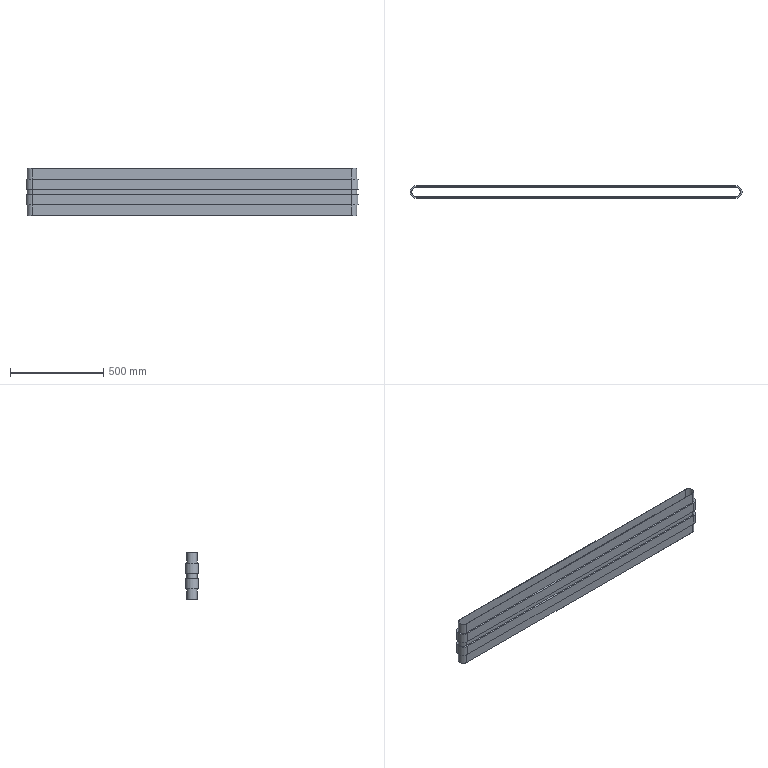Part | NX | 1 solid | 30 faces | box 1780 x 70 x 255 mm | volume 4950684 mm3 | plane 18 | cylinder 12 | commonest cylinder face diameters 54 x6 70 x4 50 x2
STEP:
#1=CARTESIAN_POINT('',(1405.,25.,-127.5));
#2=VERTEX_POINT('',#1);
#3=CARTESIAN_POINT('',(-305.,25.,-127.5));
#4=VERTEX_POINT('',#3);
#5=CARTESIAN_POINT('',(1405.,25.,-127.5));
#6=DIRECTION('',(-1.,0.,0.));
#7=VECTOR('',#6,1.);
#8=LINE('',#5,#7);
#9=EDGE_CURVE('',#2,#4,#8,.T.);
#10=ORIENTED_EDGE('',*,*,#9,.F.);
#11=CARTESIAN_POINT('',(1405.,25.,127.5));
#12=VERTEX_POINT('',#11);
#13=CARTESIAN_POINT('',(1405.,25.,-127.5));
#14=DIRECTION('',(0.,0.,1.));
#15=VECTOR('',#14,1.);
#16=LINE('',#13,#15);
#17=EDGE_CURVE('',#2,#12,#16,.T.);
#18=ORIENTED_EDGE('',*,*,#17,.T.);
#19=CARTESIAN_POINT('',(-305.,25.,127.5));
#20=VERTEX_POINT('',#19);
#21=CARTESIAN_POINT('',(1405.,25.,127.5));
#22=DIRECTION('',(-1.,0.,0.));
#23=VECTOR('',#22,1.);
#24=LINE('',#21,#23);
#25=EDGE_CURVE('',#12,#20,#24,.T.);
#26=ORIENTED_EDGE('',*,*,#25,.T.);
#27=CARTESIAN_POINT('',(-305.,25.,-127.5));
#28=DIRECTION('',(0.,0.,1.));
#29=VECTOR('',#28,1.);
#30=LINE('',#27,#29);
#31=EDGE_CURVE('',#4,#20,#30,.T.);
#32=ORIENTED_EDGE('',*,*,#31,.F.);
#33=EDGE_LOOP('',(#10,#18,#26,#32));
#34=FACE_OUTER_BOUND('',#33,.T.);
#35=CARTESIAN_POINT('',(1405.,25.,-127.5));
#36=DIRECTION('',(0.,1.,0.));
#37=DIRECTION('',(0.,0.,1.));
#38=AXIS2_PLACEMENT_3D('',#35,#36,#37);
#39=PLANE('',#38);
#40=ADVANCED_FACE('',(#34),#39,.F.);
#41=CARTESIAN_POINT('',(1405.,-25.,-127.5));
#42=VERTEX_POINT('',#41);
#43=CARTESIAN_POINT('',(1405.,0.,-127.5));
#44=DIRECTION('',(0.,0.,1.));
#45=DIRECTION('',(0.,-1.,0.));
#46=AXIS2_PLACEMENT_3D('',#43,#44,#45);
#47=CIRCLE('',#46,25.);
#48=EDGE_CURVE('',#42,#2,#47,.T.);
#49=ORIENTED_EDGE('',*,*,#48,.F.);
#50=CARTESIAN_POINT('',(1405.,-25.,127.5));
#51=VERTEX_POINT('',#50);
#52=CARTESIAN_POINT('',(1405.,-25.,-127.5));
#53=DIRECTION('',(0.,0.,1.));
#54=VECTOR('',#53,1.);
#55=LINE('',#52,#54);
#56=EDGE_CURVE('',#42,#51,#55,.T.);
#57=ORIENTED_EDGE('',*,*,#56,.T.);
#58=CARTESIAN_POINT('',(1405.,0.,127.5));
#59=DIRECTION('',(0.,0.,1.));
#60=DIRECTION('',(0.,-1.,0.));
#61=AXIS2_PLACEMENT_3D('',#58,#59,#60);
#62=CIRCLE('',#61,25.);
#63=EDGE_CURVE('',#51,#12,#62,.T.);
#64=ORIENTED_EDGE('',*,*,#63,.T.);
#65=ORIENTED_EDGE('',*,*,#17,.F.);
#66=EDGE_LOOP('',(#49,#57,#64,#65));
#67=FACE_OUTER_BOUND('',#66,.T.);
#68=CARTESIAN_POINT('',(1405.,0.,-127.5));
#69=DIRECTION('',(0.,0.,1.));
#70=DIRECTION('',(1.,0.,0.));
#71=AXIS2_PLACEMENT_3D('',#68,#69,#70);
#72=CYLINDRICAL_SURFACE('',#71,25.);
#73=ADVANCED_FACE('',(#67),#72,.F.);
#74=CARTESIAN_POINT('',(-305.,-25.,-127.5));
#75=VERTEX_POINT('',#74);
#76=CARTESIAN_POINT('',(-305.,-25.,-127.5));
#77=DIRECTION('',(1.,0.,0.));
#78=VECTOR('',#77,1.);
#79=LINE('',#76,#78);
#80=EDGE_CURVE('',#75,#42,#79,.T.);
#81=ORIENTED_EDGE('',*,*,#80,.F.);
#82=CARTESIAN_POINT('',(-305.,-25.,127.5));
#83=VERTEX_POINT('',#82);
#84=CARTESIAN_POINT('',(-305.,-25.,-127.5));
#85=DIRECTION('',(0.,0.,1.));
#86=VECTOR('',#85,1.);
#87=LINE('',#84,#86);
#88=EDGE_CURVE('',#75,#83,#87,.T.);
#89=ORIENTED_EDGE('',*,*,#88,.T.);
#90=CARTESIAN_POINT('',(-305.,-25.,127.5));
#91=DIRECTION('',(1.,0.,0.));
#92=VECTOR('',#91,1.);
#93=LINE('',#90,#92);
#94=EDGE_CURVE('',#83,#51,#93,.T.);
#95=ORIENTED_EDGE('',*,*,#94,.T.);
#96=ORIENTED_EDGE('',*,*,#56,.F.);
#97=EDGE_LOOP('',(#81,#89,#95,#96));
#98=FACE_OUTER_BOUND('',#97,.T.);
#99=CARTESIAN_POINT('',(-305.,-25.,-127.5));
#100=DIRECTION('',(0.,-1.,0.));
#101=DIRECTION('',(0.,0.,-1.));
#102=AXIS2_PLACEMENT_3D('',#99,#100,#101);
#103=PLANE('',#102);
#104=ADVANCED_FACE('',(#98),#103,.F.);
#105=CARTESIAN_POINT('',(-305.,0.,-127.5));
#106=DIRECTION('',(0.,0.,1.));
#107=DIRECTION('',(0.,1.,0.));
#108=AXIS2_PLACEMENT_3D('',#105,#106,#107);
#109=CIRCLE('',#108,25.);
#110=EDGE_CURVE('',#4,#75,#109,.T.);
#111=ORIENTED_EDGE('',*,*,#110,.F.);
#112=ORIENTED_EDGE('',*,*,#31,.T.);
#113=CARTESIAN_POINT('',(-305.,0.,127.5));
#114=DIRECTION('',(0.,0.,1.));
#115=DIRECTION('',(0.,1.,0.));
#116=AXIS2_PLACEMENT_3D('',#113,#114,#115);
#117=CIRCLE('',#116,25.);
#118=EDGE_CURVE('',#20,#83,#117,.T.);
#119=ORIENTED_EDGE('',*,*,#118,.T.);
#120=ORIENTED_EDGE('',*,*,#88,.F.);
#121=EDGE_LOOP('',(#111,#112,#119,#120));
#122=FACE_OUTER_BOUND('',#121,.T.);
#123=CARTESIAN_POINT('',(-305.,0.,-127.5));
#124=DIRECTION('',(0.,0.,1.));
#125=DIRECTION('',(1.,0.,0.));
#126=AXIS2_PLACEMENT_3D('',#123,#124,#125);
#127=CYLINDRICAL_SURFACE('',#126,25.);
#128=ADVANCED_FACE('',(#122),#127,.F.);
#129=CARTESIAN_POINT('',(1405.,-27.,-127.5));
#130=VERTEX_POINT('',#129);
#131=CARTESIAN_POINT('',(1405.,27.,-127.5));
#132=VERTEX_POINT('',#131);
#133=CARTESIAN_POINT('',(1405.,0.,-127.5));
#134=DIRECTION('',(0.,0.,1.));
#135=DIRECTION('',(0.,-1.,0.));
#136=AXIS2_PLACEMENT_3D('',#133,#134,#135);
#137=CIRCLE('',#136,27.);
#138=EDGE_CURVE('',#130,#132,#137,.T.);
#139=ORIENTED_EDGE('',*,*,#138,.F.);
#140=CARTESIAN_POINT('',(-305.,-27.,-127.5));
#141=VERTEX_POINT('',#140);
#142=CARTESIAN_POINT('',(-305.,-27.,-127.5));
#143=DIRECTION('',(1.,0.,0.));
#144=VECTOR('',#143,1.);
#145=LINE('',#142,#144);
#146=EDGE_CURVE('',#141,#130,#145,.T.);
#147=ORIENTED_EDGE('',*,*,#146,.F.);
#148=CARTESIAN_POINT('',(-305.,27.,-127.5));
#149=VERTEX_POINT('',#148);
#150=CARTESIAN_POINT('',(-305.,0.,-127.5));
#151=DIRECTION('',(0.,0.,1.));
#152=DIRECTION('',(0.,1.,0.));
#153=AXIS2_PLACEMENT_3D('',#150,#151,#152);
#154=CIRCLE('',#153,27.);
#155=EDGE_CURVE('',#149,#141,#154,.T.);
#156=ORIENTED_EDGE('',*,*,#155,.F.);
#157=CARTESIAN_POINT('',(1405.,27.,-127.5));
#158=DIRECTION('',(-1.,0.,0.));
#159=VECTOR('',#158,1.);
#160=LINE('',#157,#159);
#161=EDGE_CURVE('',#132,#149,#160,.T.);
#162=ORIENTED_EDGE('',*,*,#161,.F.);
#163=EDGE_LOOP('',(#139,#147,#156,#162));
#164=FACE_BOUND('',#163,.T.);
#165=ORIENTED_EDGE('',*,*,#110,.T.);
#166=ORIENTED_EDGE('',*,*,#80,.T.);
#167=ORIENTED_EDGE('',*,*,#48,.T.);
#168=ORIENTED_EDGE('',*,*,#9,.T.);
#169=EDGE_LOOP('',(#165,#166,#167,#168));
#170=FACE_BOUND('',#169,.T.);
#171=CARTESIAN_POINT('',(550.,26.,-127.5));
#172=DIRECTION('',(0.,0.,1.));
#173=DIRECTION('',(1.,0.,0.));
#174=AXIS2_PLACEMENT_3D('',#171,#172,#173);
#175=PLANE('',#174);
#176=ADVANCED_FACE('',(#164,#170),#175,.F.);
#177=CARTESIAN_POINT('',(-305.,27.,127.5));
#178=VERTEX_POINT('',#177);
#179=CARTESIAN_POINT('',(-305.,-27.,127.5));
#180=VERTEX_POINT('',#179);
#181=CARTESIAN_POINT('',(-305.,0.,127.5));
#182=DIRECTION('',(0.,0.,1.));
#183=DIRECTION('',(0.,1.,0.));
#184=AXIS2_PLACEMENT_3D('',#181,#182,#183);
#185=CIRCLE('',#184,27.);
#186=EDGE_CURVE('',#178,#180,#185,.T.);
#187=ORIENTED_EDGE('',*,*,#186,.T.);
#188=CARTESIAN_POINT('',(1405.,-27.,127.5));
#189=VERTEX_POINT('',#188);
#190=CARTESIAN_POINT('',(-305.,-27.,127.5));
#191=DIRECTION('',(1.,0.,0.));
#192=VECTOR('',#191,1.);
#193=LINE('',#190,#192);
#194=EDGE_CURVE('',#180,#189,#193,.T.);
#195=ORIENTED_EDGE('',*,*,#194,.T.);
#196=CARTESIAN_POINT('',(1405.,27.,127.5));
#197=VERTEX_POINT('',#196);
#198=CARTESIAN_POINT('',(1405.,0.,127.5));
#199=DIRECTION('',(0.,0.,1.));
#200=DIRECTION('',(0.,-1.,0.));
#201=AXIS2_PLACEMENT_3D('',#198,#199,#200);
#202=CIRCLE('',#201,27.);
#203=EDGE_CURVE('',#189,#197,#202,.T.);
#204=ORIENTED_EDGE('',*,*,#203,.T.);
#205=CARTESIAN_POINT('',(1405.,27.,127.5));
#206=DIRECTION('',(-1.,0.,0.));
#207=VECTOR('',#206,1.);
#208=LINE('',#205,#207);
#209=EDGE_CURVE('',#197,#178,#208,.T.);
#210=ORIENTED_EDGE('',*,*,#209,.T.);
#211=EDGE_LOOP('',(#187,#195,#204,#210));
#212=FACE_BOUND('',#211,.T.);
#213=ORIENTED_EDGE('',*,*,#63,.F.);
#214=ORIENTED_EDGE('',*,*,#94,.F.);
#215=ORIENTED_EDGE('',*,*,#118,.F.);
#216=ORIENTED_EDGE('',*,*,#25,.F.);
#217=EDGE_LOOP('',(#213,#214,#215,#216));
#218=FACE_BOUND('',#217,.T.);
#219=CARTESIAN_POINT('',(550.,26.,127.5));
#220=DIRECTION('',(0.,0.,1.));
#221=DIRECTION('',(1.,0.,0.));
#222=AXIS2_PLACEMENT_3D('',#219,#220,#221);
#223=PLANE('',#222);
#224=ADVANCED_FACE('',(#212,#218),#223,.T.);
#225=CARTESIAN_POINT('',(1405.,27.,-69.));
#226=VERTEX_POINT('',#225);
#227=CARTESIAN_POINT('',(-305.,27.,-69.));
#228=VERTEX_POINT('',#227);
#229=CARTESIAN_POINT('',(1405.,27.,-69.));
#230=DIRECTION('',(-1.,0.,0.));
#231=VECTOR('',#230,1.);
#232=LINE('',#229,#231);
#233=EDGE_CURVE('',#226,#228,#232,.T.);
#234=ORIENTED_EDGE('',*,*,#233,.F.);
#235=CARTESIAN_POINT('',(1405.,27.,-127.5));
#236=DIRECTION('',(0.,0.,1.));
#237=VECTOR('',#236,1.);
#238=LINE('',#235,#237);
#239=EDGE_CURVE('',#132,#226,#238,.T.);
#240=ORIENTED_EDGE('',*,*,#239,.F.);
#241=ORIENTED_EDGE('',*,*,#161,.T.);
#242=CARTESIAN_POINT('',(-305.,27.,-127.5));
#243=DIRECTION('',(0.,0.,1.));
#244=VECTOR('',#243,1.);
#245=LINE('',#242,#244);
#246=EDGE_CURVE('',#149,#228,#245,.T.);
#247=ORIENTED_EDGE('',*,*,#246,.T.);
#248=EDGE_LOOP('',(#234,#240,#241,#247));
#249=FACE_OUTER_BOUND('',#248,.T.);
#250=CARTESIAN_POINT('',(1405.,27.,-127.5));
#251=DIRECTION('',(0.,1.,0.));
#252=DIRECTION('',(0.,0.,1.));
#253=AXIS2_PLACEMENT_3D('',#250,#251,#252);
#254=PLANE('',#253);
#255=ADVANCED_FACE('',(#249),#254,.T.);
#256=CARTESIAN_POINT('',(1405.,27.,69.));
#257=VERTEX_POINT('',#256);
#258=CARTESIAN_POINT('',(-305.,27.,69.));
#259=VERTEX_POINT('',#258);
#260=CARTESIAN_POINT('',(1405.,27.,69.));
#261=DIRECTION('',(-1.,0.,0.));
#262=VECTOR('',#261,1.);
#263=LINE('',#260,#262);
#264=EDGE_CURVE('',#257,#259,#263,.T.);
#265=ORIENTED_EDGE('',*,*,#264,.T.);
#266=CARTESIAN_POINT('',(-305.,27.,69.));
#267=DIRECTION('',(0.,0.,1.));
#268=VECTOR('',#267,1.);
#269=LINE('',#266,#268);
#270=EDGE_CURVE('',#259,#178,#269,.T.);
#271=ORIENTED_EDGE('',*,*,#270,.T.);
#272=ORIENTED_EDGE('',*,*,#209,.F.);
#273=CARTESIAN_POINT('',(1405.,27.,69.));
#274=DIRECTION('',(0.,0.,1.));
#275=VECTOR('',#274,1.);
#276=LINE('',#273,#275);
#277=EDGE_CURVE('',#257,#197,#276,.T.);
#278=ORIENTED_EDGE('',*,*,#277,.F.);
#279=EDGE_LOOP('',(#265,#271,#272,#278));
#280=FACE_OUTER_BOUND('',#279,.T.);
#281=CARTESIAN_POINT('',(1405.,27.,-127.5));
#282=DIRECTION('',(0.,1.,0.));
#283=DIRECTION('',(0.,0.,1.));
#284=AXIS2_PLACEMENT_3D('',#281,#282,#283);
#285=PLANE('',#284);
#286=ADVANCED_FACE('',(#280),#285,.T.);
#287=CARTESIAN_POINT('',(1405.,-27.,-69.));
#288=VERTEX_POINT('',#287);
#289=CARTESIAN_POINT('',(1405.,0.,-69.));
#290=DIRECTION('',(0.,0.,1.));
#291=DIRECTION('',(0.,-1.,0.));
#292=AXIS2_PLACEMENT_3D('',#289,#290,#291);
#293=CIRCLE('',#292,27.);
#294=EDGE_CURVE('',#288,#226,#293,.T.);
#295=ORIENTED_EDGE('',*,*,#294,.F.);
#296=CARTESIAN_POINT('',(1405.,-27.,-127.5));
#297=DIRECTION('',(0.,0.,1.));
#298=VECTOR('',#297,1.);
#299=LINE('',#296,#298);
#300=EDGE_CURVE('',#130,#288,#299,.T.);
#301=ORIENTED_EDGE('',*,*,#300,.F.);
#302=ORIENTED_EDGE('',*,*,#138,.T.);
#303=ORIENTED_EDGE('',*,*,#239,.T.);
#304=EDGE_LOOP('',(#295,#301,#302,#303));
#305=FACE_OUTER_BOUND('',#304,.T.);
#306=CARTESIAN_POINT('',(1405.,0.,-127.5));
#307=DIRECTION('',(0.,0.,1.));
#308=DIRECTION('',(1.,0.,0.));
#309=AXIS2_PLACEMENT_3D('',#306,#307,#308);
#310=CYLINDRICAL_SURFACE('',#309,27.);
#311=ADVANCED_FACE('',(#305),#310,.T.);
#312=CARTESIAN_POINT('',(1405.,-27.,69.));
#313=VERTEX_POINT('',#312);
#314=CARTESIAN_POINT('',(1405.,0.,69.));
#315=DIRECTION('',(0.,0.,1.));
#316=DIRECTION('',(0.,-1.,0.));
#317=AXIS2_PLACEMENT_3D('',#314,#315,#316);
#318=CIRCLE('',#317,27.);
#319=EDGE_CURVE('',#313,#257,#318,.T.);
#320=ORIENTED_EDGE('',*,*,#319,.T.);
#321=ORIENTED_EDGE('',*,*,#277,.T.);
#322=ORIENTED_EDGE('',*,*,#203,.F.);
#323=CARTESIAN_POINT('',(1405.,-27.,69.));
#324=DIRECTION('',(0.,0.,1.));
#325=VECTOR('',#324,1.);
#326=LINE('',#323,#325);
#327=EDGE_CURVE('',#313,#189,#326,.T.);
#328=ORIENTED_EDGE('',*,*,#327,.F.);
#329=EDGE_LOOP('',(#320,#321,#322,#328));
#330=FACE_OUTER_BOUND('',#329,.T.);
#331=CARTESIAN_POINT('',(1405.,0.,-127.5));
#332=DIRECTION('',(0.,0.,1.));
#333=DIRECTION('',(1.,0.,0.));
#334=AXIS2_PLACEMENT_3D('',#331,#332,#333);
#335=CYLINDRICAL_SURFACE('',#334,27.);
#336=ADVANCED_FACE('',(#330),#335,.T.);
#337=CARTESIAN_POINT('',(-305.,-27.,-69.));
#338=VERTEX_POINT('',#337);
#339=CARTESIAN_POINT('',(-305.,-27.,-69.));
#340=DIRECTION('',(1.,0.,0.));
#341=VECTOR('',#340,1.);
#342=LINE('',#339,#341);
#343=EDGE_CURVE('',#338,#288,#342,.T.);
#344=ORIENTED_EDGE('',*,*,#343,.F.);
#345=CARTESIAN_POINT('',(-305.,-27.,-127.5));
#346=DIRECTION('',(0.,0.,1.));
#347=VECTOR('',#346,1.);
#348=LINE('',#345,#347);
#349=EDGE_CURVE('',#141,#338,#348,.T.);
#350=ORIENTED_EDGE('',*,*,#349,.F.);
#351=ORIENTED_EDGE('',*,*,#146,.T.);
#352=ORIENTED_EDGE('',*,*,#300,.T.);
#353=EDGE_LOOP('',(#344,#350,#351,#352));
#354=FACE_OUTER_BOUND('',#353,.T.);
#355=CARTESIAN_POINT('',(-305.,-27.,-127.5));
#356=DIRECTION('',(0.,-1.,0.));
#357=DIRECTION('',(0.,0.,-1.));
#358=AXIS2_PLACEMENT_3D('',#355,#356,#357);
#359=PLANE('',#358);
#360=ADVANCED_FACE('',(#354),#359,.T.);
#361=CARTESIAN_POINT('',(-305.,-27.,69.));
#362=VERTEX_POINT('',#361);
#363=CARTESIAN_POINT('',(-305.,-27.,69.));
#364=DIRECTION('',(1.,0.,0.));
#365=VECTOR('',#364,1.);
#366=LINE('',#363,#365);
#367=EDGE_CURVE('',#362,#313,#366,.T.);
#368=ORIENTED_EDGE('',*,*,#367,.T.);
#369=ORIENTED_EDGE('',*,*,#327,.T.);
#370=ORIENTED_EDGE('',*,*,#194,.F.);
#371=CARTESIAN_POINT('',(-305.,-27.,69.));
#372=DIRECTION('',(0.,0.,1.));
#373=VECTOR('',#372,1.);
#374=LINE('',#371,#373);
#375=EDGE_CURVE('',#362,#180,#374,.T.);
#376=ORIENTED_EDGE('',*,*,#375,.F.);
#377=EDGE_LOOP('',(#368,#369,#370,#376));
#378=FACE_OUTER_BOUND('',#377,.T.);
#379=CARTESIAN_POINT('',(-305.,-27.,-127.5));
#380=DIRECTION('',(0.,-1.,0.));
#381=DIRECTION('',(0.,0.,-1.));
#382=AXIS2_PLACEMENT_3D('',#379,#380,#381);
#383=PLANE('',#382);
#384=ADVANCED_FACE('',(#378),#383,.T.);
#385=CARTESIAN_POINT('',(-305.,0.,-69.));
#386=DIRECTION('',(0.,0.,1.));
#387=DIRECTION('',(0.,1.,0.));
#388=AXIS2_PLACEMENT_3D('',#385,#386,#387);
#389=CIRCLE('',#388,27.);
#390=EDGE_CURVE('',#228,#338,#389,.T.);
#391=ORIENTED_EDGE('',*,*,#390,.F.);
#392=ORIENTED_EDGE('',*,*,#246,.F.);
#393=ORIENTED_EDGE('',*,*,#155,.T.);
#394=ORIENTED_EDGE('',*,*,#349,.T.);
#395=EDGE_LOOP('',(#391,#392,#393,#394));
#396=FACE_OUTER_BOUND('',#395,.T.);
#397=CARTESIAN_POINT('',(-305.,0.,-127.5));
#398=DIRECTION('',(0.,0.,1.));
#399=DIRECTION('',(1.,0.,0.));
#400=AXIS2_PLACEMENT_3D('',#397,#398,#399);
#401=CYLINDRICAL_SURFACE('',#400,27.);
#402=ADVANCED_FACE('',(#396),#401,.T.);
#403=CARTESIAN_POINT('',(-305.,0.,69.));
#404=DIRECTION('',(0.,0.,1.));
#405=DIRECTION('',(0.,1.,0.));
#406=AXIS2_PLACEMENT_3D('',#403,#404,#405);
#407=CIRCLE('',#406,27.);
#408=EDGE_CURVE('',#259,#362,#407,.T.);
#409=ORIENTED_EDGE('',*,*,#408,.T.);
#410=ORIENTED_EDGE('',*,*,#375,.T.);
#411=ORIENTED_EDGE('',*,*,#186,.F.);
#412=ORIENTED_EDGE('',*,*,#270,.F.);
#413=EDGE_LOOP('',(#409,#410,#411,#412));
#414=FACE_OUTER_BOUND('',#413,.T.);
#415=CARTESIAN_POINT('',(-305.,0.,-127.5));
#416=DIRECTION('',(0.,0.,1.));
#417=DIRECTION('',(1.,0.,0.));
#418=AXIS2_PLACEMENT_3D('',#415,#416,#417);
#419=CYLINDRICAL_SURFACE('',#418,27.);
#420=ADVANCED_FACE('',(#414),#419,.T.);
#421=CARTESIAN_POINT('',(-305.,35.,-69.));
#422=VERTEX_POINT('',#421);
#423=CARTESIAN_POINT('',(-305.,-35.,-69.));
#424=VERTEX_POINT('',#423);
#425=CARTESIAN_POINT('',(-305.,0.,-69.));
#426=DIRECTION('',(0.,0.,1.));
#427=DIRECTION('',(0.,1.,0.));
#428=AXIS2_PLACEMENT_3D('',#425,#426,#427);
#429=CIRCLE('',#428,35.);
#430=EDGE_CURVE('',#422,#424,#429,.T.);
#431=ORIENTED_EDGE('',*,*,#430,.F.);
#432=CARTESIAN_POINT('',(1405.,35.,-69.));
#433=VERTEX_POINT('',#432);
#434=CARTESIAN_POINT('',(1405.,35.,-69.));
#435=DIRECTION('',(-1.,0.,0.));
#436=VECTOR('',#435,1.);
#437=LINE('',#434,#436);
#438=EDGE_CURVE('',#433,#422,#437,.T.);
#439=ORIENTED_EDGE('',*,*,#438,.F.);
#440=CARTESIAN_POINT('',(1405.,-35.,-69.));
#441=VERTEX_POINT('',#440);
#442=CARTESIAN_POINT('',(1405.,0.,-69.));
#443=DIRECTION('',(0.,0.,1.));
#444=DIRECTION('',(0.,-1.,0.));
#445=AXIS2_PLACEMENT_3D('',#442,#443,#444);
#446=CIRCLE('',#445,35.);
#447=EDGE_CURVE('',#441,#433,#446,.T.);
#448=ORIENTED_EDGE('',*,*,#447,.F.);
#449=CARTESIAN_POINT('',(-305.,-35.,-69.));
#450=DIRECTION('',(1.,0.,0.));
#451=VECTOR('',#450,1.);
#452=LINE('',#449,#451);
#453=EDGE_CURVE('',#424,#441,#452,.T.);
#454=ORIENTED_EDGE('',*,*,#453,.F.);
#455=EDGE_LOOP('',(#431,#439,#448,#454));
#456=FACE_BOUND('',#455,.T.);
#457=ORIENTED_EDGE('',*,*,#233,.T.);
#458=ORIENTED_EDGE('',*,*,#390,.T.);
#459=ORIENTED_EDGE('',*,*,#343,.T.);
#460=ORIENTED_EDGE('',*,*,#294,.T.);
#461=EDGE_LOOP('',(#457,#458,#459,#460));
#462=FACE_BOUND('',#461,.T.);
#463=CARTESIAN_POINT('',(0.,0.,-69.));
#464=DIRECTION('',(0.,0.,1.));
#465=DIRECTION('',(1.,0.,0.));
#466=AXIS2_PLACEMENT_3D('',#463,#464,#465);
#467=PLANE('',#466);
#468=ADVANCED_FACE('',(#456,#462),#467,.F.);
#469=CARTESIAN_POINT('',(-305.,35.,69.));
#470=VERTEX_POINT('',#469);
#471=CARTESIAN_POINT('',(-305.,-35.,69.));
#472=VERTEX_POINT('',#471);
#473=CARTESIAN_POINT('',(-305.,0.,69.));
#474=DIRECTION('',(0.,0.,1.));
#475=DIRECTION('',(0.,1.,0.));
#476=AXIS2_PLACEMENT_3D('',#473,#474,#475);
#477=CIRCLE('',#476,35.);
#478=EDGE_CURVE('',#470,#472,#477,.T.);
#479=ORIENTED_EDGE('',*,*,#478,.T.);
#480=CARTESIAN_POINT('',(1405.,-35.,69.));
#481=VERTEX_POINT('',#480);
#482=CARTESIAN_POINT('',(-305.,-35.,69.));
#483=DIRECTION('',(1.,0.,0.));
#484=VECTOR('',#483,1.);
#485=LINE('',#482,#484);
#486=EDGE_CURVE('',#472,#481,#485,.T.);
#487=ORIENTED_EDGE('',*,*,#486,.T.);
#488=CARTESIAN_POINT('',(1405.,35.,69.));
#489=VERTEX_POINT('',#488);
#490=CARTESIAN_POINT('',(1405.,0.,69.));
#491=DIRECTION('',(0.,0.,1.));
#492=DIRECTION('',(0.,-1.,0.));
#493=AXIS2_PLACEMENT_3D('',#490,#491,#492);
#494=CIRCLE('',#493,35.);
#495=EDGE_CURVE('',#481,#489,#494,.T.);
#496=ORIENTED_EDGE('',*,*,#495,.T.);
#497=CARTESIAN_POINT('',(1405.,35.,69.));
#498=DIRECTION('',(-1.,0.,0.));
#499=VECTOR('',#498,1.);
#500=LINE('',#497,#499);
#501=EDGE_CURVE('',#489,#470,#500,.T.);
#502=ORIENTED_EDGE('',*,*,#501,.T.);
#503=EDGE_LOOP('',(#479,#487,#496,#502));
#504=FACE_BOUND('',#503,.T.);
#505=ORIENTED_EDGE('',*,*,#264,.F.);
#506=ORIENTED_EDGE('',*,*,#319,.F.);
#507=ORIENTED_EDGE('',*,*,#367,.F.);
#508=ORIENTED_EDGE('',*,*,#408,.F.);
#509=EDGE_LOOP('',(#505,#506,#507,#508));
#510=FACE_BOUND('',#509,.T.);
#511=CARTESIAN_POINT('',(0.,0.,69.));
#512=DIRECTION('',(0.,0.,1.));
#513=DIRECTION('',(1.,0.,0.));
#514=AXIS2_PLACEMENT_3D('',#511,#512,#513);
#515=PLANE('',#514);
#516=ADVANCED_FACE('',(#504,#510),#515,.T.);
#517=CARTESIAN_POINT('',(-305.,35.,-15.));
#518=VERTEX_POINT('',#517);
#519=CARTESIAN_POINT('',(-305.,-35.,-15.));
#520=VERTEX_POINT('',#519);
#521=CARTESIAN_POINT('',(-305.,0.,-15.));
#522=DIRECTION('',(0.,0.,1.));
#523=DIRECTION('',(0.,1.,0.));
#524=AXIS2_PLACEMENT_3D('',#521,#522,#523);
#525=CIRCLE('',#524,35.);
#526=EDGE_CURVE('',#518,#520,#525,.T.);
#527=ORIENTED_EDGE('',*,*,#526,.F.);
#528=CARTESIAN_POINT('',(-305.,35.,-69.));
#529=DIRECTION('',(0.,0.,1.));
#530=VECTOR('',#529,1.);
#531=LINE('',#528,#530);
#532=EDGE_CURVE('',#422,#518,#531,.T.);
#533=ORIENTED_EDGE('',*,*,#532,.F.);
#534=ORIENTED_EDGE('',*,*,#430,.T.);
#535=CARTESIAN_POINT('',(-305.,-35.,-69.));
#536=DIRECTION('',(0.,0.,1.));
#537=VECTOR('',#536,1.);
#538=LINE('',#535,#537);
#539=EDGE_CURVE('',#424,#520,#538,.T.);
#540=ORIENTED_EDGE('',*,*,#539,.T.);
#541=EDGE_LOOP('',(#527,#533,#534,#540));
#542=FACE_OUTER_BOUND('',#541,.T.);
#543=CARTESIAN_POINT('',(-305.,0.,-69.));
#544=DIRECTION('',(0.,0.,1.));
#545=DIRECTION('',(1.,0.,0.));
#546=AXIS2_PLACEMENT_3D('',#543,#544,#545);
#547=CYLINDRICAL_SURFACE('',#546,35.);
#548=ADVANCED_FACE('',(#542),#547,.T.);
#549=CARTESIAN_POINT('',(-305.,35.,15.));
#550=VERTEX_POINT('',#549);
#551=CARTESIAN_POINT('',(-305.,-35.,15.));
#552=VERTEX_POINT('',#551);
#553=CARTESIAN_POINT('',(-305.,0.,15.));
#554=DIRECTION('',(0.,0.,1.));
#555=DIRECTION('',(0.,1.,0.));
#556=AXIS2_PLACEMENT_3D('',#553,#554,#555);
#557=CIRCLE('',#556,35.);
#558=EDGE_CURVE('',#550,#552,#557,.T.);
#559=ORIENTED_EDGE('',*,*,#558,.T.);
#560=CARTESIAN_POINT('',(-305.,-35.,15.));
#561=DIRECTION('',(0.,0.,1.));
#562=VECTOR('',#561,1.);
#563=LINE('',#560,#562);
#564=EDGE_CURVE('',#552,#472,#563,.T.);
#565=ORIENTED_EDGE('',*,*,#564,.T.);
#566=ORIENTED_EDGE('',*,*,#478,.F.);
#567=CARTESIAN_POINT('',(-305.,35.,15.));
#568=DIRECTION('',(0.,0.,1.));
#569=VECTOR('',#568,1.);
#570=LINE('',#567,#569);
#571=EDGE_CURVE('',#550,#470,#570,.T.);
#572=ORIENTED_EDGE('',*,*,#571,.F.);
#573=EDGE_LOOP('',(#559,#565,#566,#572));
#574=FACE_OUTER_BOUND('',#573,.T.);
#575=CARTESIAN_POINT('',(-305.,0.,-69.));
#576=DIRECTION('',(0.,0.,1.));
#577=DIRECTION('',(1.,0.,0.));
#578=AXIS2_PLACEMENT_3D('',#575,#576,#577);
#579=CYLINDRICAL_SURFACE('',#578,35.);
#580=ADVANCED_FACE('',(#574),#579,.T.);
#581=CARTESIAN_POINT('',(1405.,-35.,-15.));
#582=VERTEX_POINT('',#581);
#583=CARTESIAN_POINT('',(-305.,-35.,-15.));
#584=DIRECTION('',(1.,0.,0.));
#585=VECTOR('',#584,1.);
#586=LINE('',#583,#585);
#587=EDGE_CURVE('',#520,#582,#586,.T.);
#588=ORIENTED_EDGE('',*,*,#587,.F.);
#589=ORIENTED_EDGE('',*,*,#539,.F.);
#590=ORIENTED_EDGE('',*,*,#453,.T.);
#591=CARTESIAN_POINT('',(1405.,-35.,-69.));
#592=DIRECTION('',(0.,0.,1.));
#593=VECTOR('',#592,1.);
#594=LINE('',#591,#593);
#595=EDGE_CURVE('',#441,#582,#594,.T.);
#596=ORIENTED_EDGE('',*,*,#595,.T.);
#597=EDGE_LOOP('',(#588,#589,#590,#596));
#598=FACE_OUTER_BOUND('',#597,.T.);
#599=CARTESIAN_POINT('',(-305.,-35.,-69.));
#600=DIRECTION('',(0.,-1.,0.));
#601=DIRECTION('',(0.,0.,-1.));
#602=AXIS2_PLACEMENT_3D('',#599,#600,#601);
#603=PLANE('',#602);
#604=ADVANCED_FACE('',(#598),#603,.T.);
#605=CARTESIAN_POINT('',(1405.,-35.,15.));
#606=VERTEX_POINT('',#605);
#607=CARTESIAN_POINT('',(-305.,-35.,15.));
#608=DIRECTION('',(1.,0.,0.));
#609=VECTOR('',#608,1.);
#610=LINE('',#607,#609);
#611=EDGE_CURVE('',#552,#606,#610,.T.);
#612=ORIENTED_EDGE('',*,*,#611,.T.);
#613=CARTESIAN_POINT('',(1405.,-35.,15.));
#614=DIRECTION('',(0.,0.,1.));
#615=VECTOR('',#614,1.);
#616=LINE('',#613,#615);
#617=EDGE_CURVE('',#606,#481,#616,.T.);
#618=ORIENTED_EDGE('',*,*,#617,.T.);
#619=ORIENTED_EDGE('',*,*,#486,.F.);
#620=ORIENTED_EDGE('',*,*,#564,.F.);
#621=EDGE_LOOP('',(#612,#618,#619,#620));
#622=FACE_OUTER_BOUND('',#621,.T.);
#623=CARTESIAN_POINT('',(-305.,-35.,-69.));
#624=DIRECTION('',(0.,-1.,0.));
#625=DIRECTION('',(0.,0.,-1.));
#626=AXIS2_PLACEMENT_3D('',#623,#624,#625);
#627=PLANE('',#626);
#628=ADVANCED_FACE('',(#622),#627,.T.);
#629=CARTESIAN_POINT('',(1405.,35.,-15.));
#630=VERTEX_POINT('',#629);
#631=CARTESIAN_POINT('',(1405.,0.,-15.));
#632=DIRECTION('',(0.,0.,1.));
#633=DIRECTION('',(0.,-1.,0.));
#634=AXIS2_PLACEMENT_3D('',#631,#632,#633);
#635=CIRCLE('',#634,35.);
#636=EDGE_CURVE('',#582,#630,#635,.T.);
#637=ORIENTED_EDGE('',*,*,#636,.F.);
#638=ORIENTED_EDGE('',*,*,#595,.F.);
#639=ORIENTED_EDGE('',*,*,#447,.T.);
#640=CARTESIAN_POINT('',(1405.,35.,-69.));
#641=DIRECTION('',(0.,0.,1.));
#642=VECTOR('',#641,1.);
#643=LINE('',#640,#642);
#644=EDGE_CURVE('',#433,#630,#643,.T.);
#645=ORIENTED_EDGE('',*,*,#644,.T.);
#646=EDGE_LOOP('',(#637,#638,#639,#645));
#647=FACE_OUTER_BOUND('',#646,.T.);
#648=CARTESIAN_POINT('',(1405.,0.,-69.));
#649=DIRECTION('',(0.,0.,1.));
#650=DIRECTION('',(1.,0.,0.));
#651=AXIS2_PLACEMENT_3D('',#648,#649,#650);
#652=CYLINDRICAL_SURFACE('',#651,35.);
#653=ADVANCED_FACE('',(#647),#652,.T.);
#654=CARTESIAN_POINT('',(1405.,35.,15.));
#655=VERTEX_POINT('',#654);
#656=CARTESIAN_POINT('',(1405.,0.,15.));
#657=DIRECTION('',(0.,0.,1.));
#658=DIRECTION('',(0.,-1.,0.));
#659=AXIS2_PLACEMENT_3D('',#656,#657,#658);
#660=CIRCLE('',#659,35.);
#661=EDGE_CURVE('',#606,#655,#660,.T.);
#662=ORIENTED_EDGE('',*,*,#661,.T.);
#663=CARTESIAN_POINT('',(1405.,35.,15.));
#664=DIRECTION('',(0.,0.,1.));
#665=VECTOR('',#664,1.);
#666=LINE('',#663,#665);
#667=EDGE_CURVE('',#655,#489,#666,.T.);
#668=ORIENTED_EDGE('',*,*,#667,.T.);
#669=ORIENTED_EDGE('',*,*,#495,.F.);
#670=ORIENTED_EDGE('',*,*,#617,.F.);
#671=EDGE_LOOP('',(#662,#668,#669,#670));
#672=FACE_OUTER_BOUND('',#671,.T.);
#673=CARTESIAN_POINT('',(1405.,0.,-69.));
#674=DIRECTION('',(0.,0.,1.));
#675=DIRECTION('',(1.,0.,0.));
#676=AXIS2_PLACEMENT_3D('',#673,#674,#675);
#677=CYLINDRICAL_SURFACE('',#676,35.);
#678=ADVANCED_FACE('',(#672),#677,.T.);
#679=CARTESIAN_POINT('',(1405.,35.,-15.));
#680=DIRECTION('',(-1.,0.,0.));
#681=VECTOR('',#680,1.);
#682=LINE('',#679,#681);
#683=EDGE_CURVE('',#630,#518,#682,.T.);
#684=ORIENTED_EDGE('',*,*,#683,.F.);
#685=ORIENTED_EDGE('',*,*,#644,.F.);
#686=ORIENTED_EDGE('',*,*,#438,.T.);
#687=ORIENTED_EDGE('',*,*,#532,.T.);
#688=EDGE_LOOP('',(#684,#685,#686,#687));
#689=FACE_OUTER_BOUND('',#688,.T.);
#690=CARTESIAN_POINT('',(1405.,35.,-69.));
#691=DIRECTION('',(0.,1.,0.));
#692=DIRECTION('',(0.,0.,1.));
#693=AXIS2_PLACEMENT_3D('',#690,#691,#692);
#694=PLANE('',#693);
#695=ADVANCED_FACE('',(#689),#694,.T.);
#696=CARTESIAN_POINT('',(1405.,35.,15.));
#697=DIRECTION('',(-1.,0.,0.));
#698=VECTOR('',#697,1.);
#699=LINE('',#696,#698);
#700=EDGE_CURVE('',#655,#550,#699,.T.);
#701=ORIENTED_EDGE('',*,*,#700,.T.);
#702=ORIENTED_EDGE('',*,*,#571,.T.);
#703=ORIENTED_EDGE('',*,*,#501,.F.);
#704=ORIENTED_EDGE('',*,*,#667,.F.);
#705=EDGE_LOOP('',(#701,#702,#703,#704));
#706=FACE_OUTER_BOUND('',#705,.T.);
#707=CARTESIAN_POINT('',(1405.,35.,-69.));
#708=DIRECTION('',(0.,1.,0.));
#709=DIRECTION('',(0.,0.,1.));
#710=AXIS2_PLACEMENT_3D('',#707,#708,#709);
#711=PLANE('',#710);
#712=ADVANCED_FACE('',(#706),#711,.T.);
#713=ORIENTED_EDGE('',*,*,#526,.T.);
#714=ORIENTED_EDGE('',*,*,#587,.T.);
#715=ORIENTED_EDGE('',*,*,#636,.T.);
#716=ORIENTED_EDGE('',*,*,#683,.T.);
#717=EDGE_LOOP('',(#713,#714,#715,#716));
#718=FACE_BOUND('',#717,.T.);
#719=CARTESIAN_POINT('',(1405.,-27.,-15.));
#720=VERTEX_POINT('',#719);
#721=CARTESIAN_POINT('',(1405.,27.,-15.));
#722=VERTEX_POINT('',#721);
#723=CARTESIAN_POINT('',(1405.,0.,-15.));
#724=DIRECTION('',(0.,0.,1.));
#725=DIRECTION('',(0.,-1.,0.));
#726=AXIS2_PLACEMENT_3D('',#723,#724,#725);
#727=CIRCLE('',#726,27.);
#728=EDGE_CURVE('',#720,#722,#727,.T.);
#729=ORIENTED_EDGE('',*,*,#728,.F.);
#730=CARTESIAN_POINT('',(-305.,-27.,-15.));
#731=VERTEX_POINT('',#730);
#732=CARTESIAN_POINT('',(-305.,-27.,-15.));
#733=DIRECTION('',(1.,0.,0.));
#734=VECTOR('',#733,1.);
#735=LINE('',#732,#734);
#736=EDGE_CURVE('',#731,#720,#735,.T.);
#737=ORIENTED_EDGE('',*,*,#736,.F.);
#738=CARTESIAN_POINT('',(-305.,27.,-15.));
#739=VERTEX_POINT('',#738);
#740=CARTESIAN_POINT('',(-305.,0.,-15.));
#741=DIRECTION('',(0.,0.,1.));
#742=DIRECTION('',(0.,1.,0.));
#743=AXIS2_PLACEMENT_3D('',#740,#741,#742);
#744=CIRCLE('',#743,27.);
#745=EDGE_CURVE('',#739,#731,#744,.T.);
#746=ORIENTED_EDGE('',*,*,#745,.F.);
#747=CARTESIAN_POINT('',(1405.,27.,-15.));
#748=DIRECTION('',(-1.,0.,0.));
#749=VECTOR('',#748,1.);
#750=LINE('',#747,#749);
#751=EDGE_CURVE('',#722,#739,#750,.T.);
#752=ORIENTED_EDGE('',*,*,#751,.F.);
#753=EDGE_LOOP('',(#729,#737,#746,#752));
#754=FACE_BOUND('',#753,.T.);
#755=CARTESIAN_POINT('',(0.,0.,-15.));
#756=DIRECTION('',(0.,0.,1.));
#757=DIRECTION('',(1.,0.,0.));
#758=AXIS2_PLACEMENT_3D('',#755,#756,#757);
#759=PLANE('',#758);
#760=ADVANCED_FACE('',(#718,#754),#759,.T.);
#761=ORIENTED_EDGE('',*,*,#558,.F.);
#762=ORIENTED_EDGE('',*,*,#700,.F.);
#763=ORIENTED_EDGE('',*,*,#661,.F.);
#764=ORIENTED_EDGE('',*,*,#611,.F.);
#765=EDGE_LOOP('',(#761,#762,#763,#764));
#766=FACE_BOUND('',#765,.T.);
#767=CARTESIAN_POINT('',(1405.,-27.,15.));
#768=VERTEX_POINT('',#767);
#769=CARTESIAN_POINT('',(1405.,27.,15.));
#770=VERTEX_POINT('',#769);
#771=CARTESIAN_POINT('',(1405.,0.,15.));
#772=DIRECTION('',(0.,0.,1.));
#773=DIRECTION('',(0.,-1.,0.));
#774=AXIS2_PLACEMENT_3D('',#771,#772,#773);
#775=CIRCLE('',#774,27.);
#776=EDGE_CURVE('',#768,#770,#775,.T.);
#777=ORIENTED_EDGE('',*,*,#776,.T.);
#778=CARTESIAN_POINT('',(-305.,27.,15.));
#779=VERTEX_POINT('',#778);
#780=CARTESIAN_POINT('',(1405.,27.,15.));
#781=DIRECTION('',(-1.,0.,0.));
#782=VECTOR('',#781,1.);
#783=LINE('',#780,#782);
#784=EDGE_CURVE('',#770,#779,#783,.T.);
#785=ORIENTED_EDGE('',*,*,#784,.T.);
#786=CARTESIAN_POINT('',(-305.,-27.,15.));
#787=VERTEX_POINT('',#786);
#788=CARTESIAN_POINT('',(-305.,0.,15.));
#789=DIRECTION('',(0.,0.,1.));
#790=DIRECTION('',(0.,1.,0.));
#791=AXIS2_PLACEMENT_3D('',#788,#789,#790);
#792=CIRCLE('',#791,27.);
#793=EDGE_CURVE('',#779,#787,#792,.T.);
#794=ORIENTED_EDGE('',*,*,#793,.T.);
#795=CARTESIAN_POINT('',(-305.,-27.,15.));
#796=DIRECTION('',(1.,0.,0.));
#797=VECTOR('',#796,1.);
#798=LINE('',#795,#797);
#799=EDGE_CURVE('',#787,#768,#798,.T.);
#800=ORIENTED_EDGE('',*,*,#799,.T.);
#801=EDGE_LOOP('',(#777,#785,#794,#800));
#802=FACE_BOUND('',#801,.T.);
#803=CARTESIAN_POINT('',(0.,0.,15.));
#804=DIRECTION('',(0.,0.,1.));
#805=DIRECTION('',(1.,0.,0.));
#806=AXIS2_PLACEMENT_3D('',#803,#804,#805);
#807=PLANE('',#806);
#808=ADVANCED_FACE('',(#766,#802),#807,.F.);
#809=ORIENTED_EDGE('',*,*,#728,.T.);
#810=CARTESIAN_POINT('',(1405.,27.,15.));
#811=DIRECTION('',(0.,0.,-1.));
#812=VECTOR('',#811,1.);
#813=LINE('',#810,#812);
#814=EDGE_CURVE('',#770,#722,#813,.T.);
#815=ORIENTED_EDGE('',*,*,#814,.F.);
#816=ORIENTED_EDGE('',*,*,#776,.F.);
#817=CARTESIAN_POINT('',(1405.,-27.,15.));
#818=DIRECTION('',(0.,0.,-1.));
#819=VECTOR('',#818,1.);
#820=LINE('',#817,#819);
#821=EDGE_CURVE('',#768,#720,#820,.T.);
#822=ORIENTED_EDGE('',*,*,#821,.T.);
#823=EDGE_LOOP('',(#809,#815,#816,#822));
#824=FACE_OUTER_BOUND('',#823,.T.);
#825=CARTESIAN_POINT('',(1405.,0.,-15.));
#826=DIRECTION('',(0.,0.,1.));
#827=DIRECTION('',(1.,0.,0.));
#828=AXIS2_PLACEMENT_3D('',#825,#826,#827);
#829=CYLINDRICAL_SURFACE('',#828,27.);
#830=ADVANCED_FACE('',(#824),#829,.T.);
#831=ORIENTED_EDGE('',*,*,#736,.T.);
#832=ORIENTED_EDGE('',*,*,#821,.F.);
#833=ORIENTED_EDGE('',*,*,#799,.F.);
#834=CARTESIAN_POINT('',(-305.,-27.,15.));
#835=DIRECTION('',(0.,0.,-1.));
#836=VECTOR('',#835,1.);
#837=LINE('',#834,#836);
#838=EDGE_CURVE('',#787,#731,#837,.T.);
#839=ORIENTED_EDGE('',*,*,#838,.T.);
#840=EDGE_LOOP('',(#831,#832,#833,#839));
#841=FACE_OUTER_BOUND('',#840,.T.);
#842=CARTESIAN_POINT('',(1405.,-27.,-15.));
#843=DIRECTION('',(0.,1.,0.));
#844=DIRECTION('',(0.,0.,1.));
#845=AXIS2_PLACEMENT_3D('',#842,#843,#844);
#846=PLANE('',#845);
#847=ADVANCED_FACE('',(#841),#846,.F.);
#848=ORIENTED_EDGE('',*,*,#745,.T.);
#849=ORIENTED_EDGE('',*,*,#838,.F.);
#850=ORIENTED_EDGE('',*,*,#793,.F.);
#851=CARTESIAN_POINT('',(-305.,27.,15.));
#852=DIRECTION('',(0.,0.,-1.));
#853=VECTOR('',#852,1.);
#854=LINE('',#851,#853);
#855=EDGE_CURVE('',#779,#739,#854,.T.);
#856=ORIENTED_EDGE('',*,*,#855,.T.);
#857=EDGE_LOOP('',(#848,#849,#850,#856));
#858=FACE_OUTER_BOUND('',#857,.T.);
#859=CARTESIAN_POINT('',(-305.,0.,-15.));
#860=DIRECTION('',(0.,0.,1.));
#861=DIRECTION('',(1.,0.,0.));
#862=AXIS2_PLACEMENT_3D('',#859,#860,#861);
#863=CYLINDRICAL_SURFACE('',#862,27.);
#864=ADVANCED_FACE('',(#858),#863,.T.);
#865=ORIENTED_EDGE('',*,*,#751,.T.);
#866=ORIENTED_EDGE('',*,*,#855,.F.);
#867=ORIENTED_EDGE('',*,*,#784,.F.);
#868=ORIENTED_EDGE('',*,*,#814,.T.);
#869=EDGE_LOOP('',(#865,#866,#867,#868));
#870=FACE_OUTER_BOUND('',#869,.T.);
#871=CARTESIAN_POINT('',(-305.,27.,-15.));
#872=DIRECTION('',(0.,-1.,0.));
#873=DIRECTION('',(0.,0.,-1.));
#874=AXIS2_PLACEMENT_3D('',#871,#872,#873);
#875=PLANE('',#874);
#876=ADVANCED_FACE('',(#870),#875,.F.);
#877=CLOSED_SHELL('',(#40,#73,#104,#128,#176,#224,#255,#286,#311,#336,#360,#384,#402,#420,#468,#516,#548,#580,#604,#628,#653,#678,#695,#712,#760,#808,#830,#847,#864,#876));
#878=MANIFOLD_SOLID_BREP('',#877);
#879=(LENGTH_UNIT()NAMED_UNIT(*)SI_UNIT(.MILLI.,.METRE.));
#880=UNCERTAINTY_MEASURE_WITH_UNIT(LENGTH_MEASURE(0.00002),#879,'','');
#881=(NAMED_UNIT(*)PLANE_ANGLE_UNIT()SI_UNIT($,.RADIAN.));
#882=PLANE_ANGLE_MEASURE_WITH_UNIT(PLANE_ANGLE_MEASURE(0.01745),#881);
#883=DIMENSIONAL_EXPONENTS(0.,0.,0.,0.,0.,0.,0.);
#884=(CONVERSION_BASED_UNIT('DEGREE',#882)NAMED_UNIT(#883)PLANE_ANGLE_UNIT());
#885=(NAMED_UNIT(*)SI_UNIT($,.STERADIAN.)SOLID_ANGLE_UNIT());
#886=(GEOMETRIC_REPRESENTATION_CONTEXT(3)GLOBAL_UNCERTAINTY_ASSIGNED_CONTEXT((#880))GLOBAL_UNIT_ASSIGNED_CONTEXT((#879,#884,#885))REPRESENTATION_CONTEXT('',''));
#887=ADVANCED_BREP_SHAPE_REPRESENTATION('',(#878),#886);